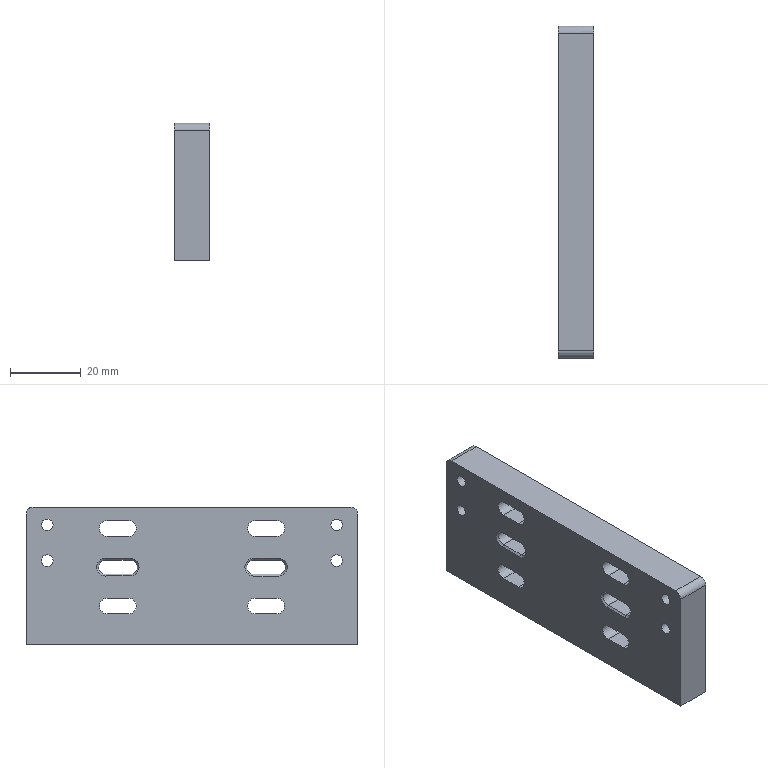CAM job | NX | 3+2 milling, drilling | part box 10.067 x 94 x 39 mm | stock box 12.07 x 99.016 x 44 mm
Tools:
number,name,description,diameter,corner_radius,flute_length,length,flutes
3,D3,平底铣刀-粗,3.0,0.0,20.0,75.0,2
6,D6,平底铣刀-粗,6.0,0.0,25.0,75.0,2
9,D10,平底铣刀-粗,10.0,0.0,35.0,75.0,2
11,D3-J,平底铣刀-精,3.0,0.0,50.0,75.0,2
7,D6-J,平底铣刀-精,6.0,0.0,25.0,75.0,2
10,D10-J,平底铣刀-精,10.0,0.0,35.0,75.0,2
1,D80R0.8飞刀,圆鼻刀-粗,80.0,0.8,50.0,75.0,2
1,D80R0.8飞刀-J,圆鼻刀-精,80.0,0.8,50.0,75.0,2
2,D6倒角刀,倒角刀,6.0,0.0,3.0,25.0,2
21,M4X0.7,丝锥,3.3,0.0,35.0,50.0,2
13,钻头3.3,Twist Drill 3.3 mm,3.3,0.0,35.0,35.008,2
Operations:
program,operation,operation_type,tool,method,geometry_group,spindle_rpm,surface_speed,feed_per_tooth,feed_cut,feed_plunge,cut_length_mm,path_length_mm,cut_time_min,machine_time_min
B,BOTTOMWALL_FACEMILL_ROUGH_COPY,VolumeBased25DMillingOperation,D80R0.8飞刀,LAYERROUGH-DEPTHK-STEPG,W-B,2800.0,703.696,0.5357,3000.0,100.0,808.874,1437.906,0.2696,0.3325
B,BOTTOMWALL_FACEMILL_FINISH_COPY,VolumeBased25DMillingOperation,D80R0.8飞刀-J,SIDEFINISH-DEPTHK-STEPG,W-B,4000.0,1005.28,0.125,1000.0,100.0,202.022,238.022,0.202,0.2056
B,DRILLCHAMFER_2,Operation,D6倒角刀,METHOD,W-B,8000.0,150.796,0.0625,1000.0,0.0,20.8,193.822,0.0208,0.0381
B,PLANARDEBURR_6X45L_COPY,SurfaceContour,D6倒角刀,WALLCLIMB_CHAMFER-DEPTH0-STEPG,W-B,6500.0,122.519,0.1154,1500.0,100.0,401.019,767.306,0.2673,0.304
B,C0.3_CLOSEDCONTOURCHAMFER_6X45L_COPY_1,PlanarMilling,D6倒角刀,WALLCLIMB_CHAMFER-DEPTH0-STEPG,W-B,7000.0,131.0,0.0714,1000.0,100.0,71.974,194.702,0.072,0.0842
A,TOPFACE,FaceMilling,D80R0.8飞刀,SIDEFINISH-DEPTHK-STEPG,W-A,4000.0,1005.31,0.125,1000.0,100.0,188.007,224.007,0.188,0.1916
A,PROFILE_ROUGH_2,VolumeBased25DMillingOperation,D10,METHOD,W-A,8000.0,251.327,0.3125,5000.0,80.0,4446.639,4495.239,0.8893,0.8942
A,SPOTDRILL-DEPTH0.8,Operation,D6倒角刀,NONE,W-A,8000.0,150.796,0.0312,500.0,90.0,7.2,159.804,0.0144,0.0297
A,THRUHOLE-M4TAPDRILL,Operation,钻头3.3,NONE,W-A,3000.0,31.102,0.05,300.0,90.0,67.966,281.335,0.2266,0.2479
A,BLINDSLOT_ROUGH,VolumeBased25DMillingOperation,D6,METHOD,W-A,6000.0,113.0,0.2083,2500.0,100.0,2054.087,2317.198,0.8216,0.8479
A,SLOT_ROUGH_2,VolumeBased25DMillingOperation,D3,METHOD,W-A,6000.0,56.549,0.125,1500.0,100.0,4040.037,4344.348,2.693,2.724
A,SLOT_ROUGH_2_COPY,VolumeBased25DMillingOperation,D3,METHOD,W-A,6000.0,56.549,0.125,1500.0,100.0,3755.583,3896.083,2.504,2.518
A,SLOT_FINISH,VolumeBased25DMillingOperation,D6-J,METHOD,W-A,6000.0,113.0,0.0667,600.0,100.0,82.046,367.957,0.1367,0.1653
A,SLOT_FINISH_4,VolumeBased25DMillingOperation,D3-J,METHOD,W-A,6000.0,113.0,0.0417,500.0,100.0,152.028,505.179,0.3041,0.3394
A,SOLIDONLY,SurfaceContour,D6倒角刀,METHOD,W-A,8000.0,150.796,0.1875,3000.0,100.0,281.602,317.403,0.0939,0.0974
A,DRILLCHAMFER_1,Operation,D6倒角刀,METHOD,W-A,8000.0,150.796,0.0312,500.0,0.0,20.8,193.822,0.0416,0.0589
A,BOTTOMWALL_CHAMFER_COPY,VolumeBased25DMillingOperation,D6倒角刀,WALLCLIMB_CHAMFER-DEPTH0-STEPG,W-A,6500.0,122.519,0.1154,1500.0,100.0,161.312,411.578,0.1075,0.1326
A,C0.3_CLOSEDCONTOURCHAMFER_6X45L_COPY,PlanarMilling,D6倒角刀,WALLCLIMB_CHAMFER-DEPTH0-STEPG,W-A,7000.0,131.0,0.1071,1500.0,100.0,71.974,194.702,0.048,0.0603
A,SLOT_FINISH_3,VolumeBased25DMillingOperation,D3-J,METHOD,W-A,6000.0,113.0,0.0417,500.0,100.0,116.597,311.296,0.2332,0.2527
A,THRUHOLE-TAPM4,Operation,M4X0.7,METHOD,W-A,600.0,6.22,0.0006,0.7,90.0,56.0,257.404,80.0,80.02
A,PROFILE_SEMIFINISH_2,VolumeBased25DMillingOperation,D10-J,METHOD,W-A,8000.0,251.327,0.0625,1000.0,100.0,300.671,359.872,0.3007,0.3066